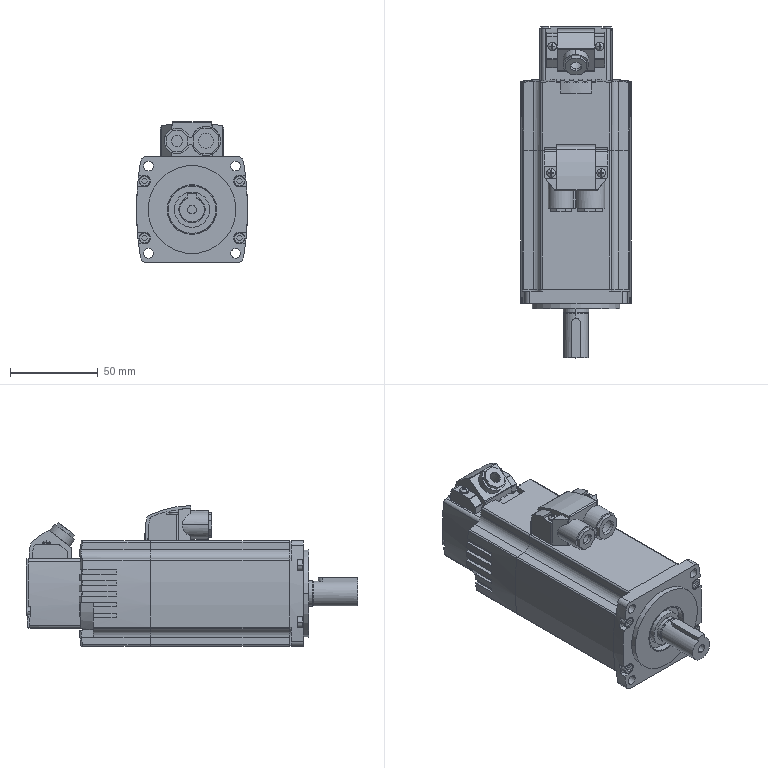Part | STEP file | 8 solids | 755 faces | box 63.062 x 188.688 x 80 mm | volume 431476 mm3 | plane 453 | cylinder 248 | torus 28 | sphere 18 | other 8 | commonest cylinder face diameters 2 x24 1.2 x23 5 x12 9.4 x12 2.8 x8 3.2 x8